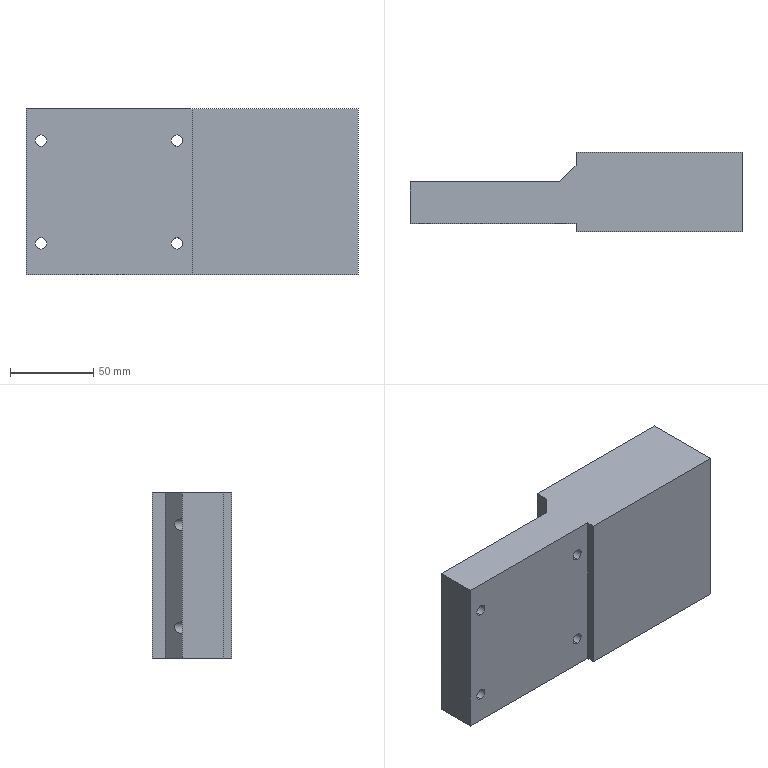Part | STEP file | HXGR200008-05-11 | 1 solid | 35 faces | box 200 x 48 x 100 mm | volume 720235 mm3 | cylinder 16 | plane 11 | cone 8 | commonest cylinder face diameters 6.8 x8 10.2 x8
STEP:
#1=CARTESIAN_POINT('',(115.,15.25,-40.1));
#2=VERTEX_POINT('',#1);
#3=CARTESIAN_POINT('',(115.,15.25,-29.9));
#4=VERTEX_POINT('',#3);
#5=CARTESIAN_POINT('',(115.,15.25,-35.));
#6=DIRECTION('',(0.,1.,0.));
#7=DIRECTION('',(0.,0.,1.));
#8=AXIS2_PLACEMENT_3D('',#5,#6,#7);
#9=CIRCLE('',#8,5.1);
#10=EDGE_CURVE('',#2,#4,#9,.T.);
#11=ORIENTED_EDGE('',*,*,#10,.F.);
#12=CARTESIAN_POINT('',(115.,48.,-40.1));
#13=VERTEX_POINT('',#12);
#14=CARTESIAN_POINT('',(115.,48.,-40.1));
#15=DIRECTION('',(0.,1.,0.));
#16=VECTOR('',#15,1000.);
#17=LINE('',#14,#16);
#18=EDGE_CURVE('',#2,#13,#17,.T.);
#19=ORIENTED_EDGE('',*,*,#18,.T.);
#20=CARTESIAN_POINT('',(115.,48.,-29.9));
#21=VERTEX_POINT('',#20);
#22=CARTESIAN_POINT('',(115.,48.,-35.));
#23=DIRECTION('',(0.,1.,0.));
#24=DIRECTION('',(0.,0.,1.));
#25=AXIS2_PLACEMENT_3D('',#22,#23,#24);
#26=CIRCLE('',#25,5.1);
#27=EDGE_CURVE('',#13,#21,#26,.T.);
#28=ORIENTED_EDGE('',*,*,#27,.T.);
#29=CARTESIAN_POINT('',(115.,48.,-29.9));
#30=DIRECTION('',(0.,1.,0.));
#31=VECTOR('',#30,1000.);
#32=LINE('',#29,#31);
#33=EDGE_CURVE('',#4,#21,#32,.T.);
#34=ORIENTED_EDGE('',*,*,#33,.F.);
#35=EDGE_LOOP('',(#11,#19,#28,#34));
#36=FACE_OUTER_BOUND('',#35,.T.);
#37=CARTESIAN_POINT('',(115.,48.,-35.));
#38=DIRECTION('',(0.,1.,0.));
#39=DIRECTION('',(0.,0.,1.));
#40=AXIS2_PLACEMENT_3D('',#37,#38,#39);
#41=CYLINDRICAL_SURFACE('',#40,5.1);
#42=ADVANCED_FACE('',(#36),#41,.F.);
#43=CARTESIAN_POINT('',(115.,12.186,-35.));
#44=VERTEX_POINT('',#43);
#45=CARTESIAN_POINT('',(115.,15.25,-29.9));
#46=DIRECTION('',(0.,0.515,0.8572));
#47=VECTOR('',#46,1000.);
#48=LINE('',#45,#47);
#49=EDGE_CURVE('',#44,#4,#48,.T.);
#50=ORIENTED_EDGE('',*,*,#49,.F.);
#51=CARTESIAN_POINT('',(115.,15.25,-40.1));
#52=DIRECTION('',(0.,0.515,-0.8572));
#53=VECTOR('',#52,1000.);
#54=LINE('',#51,#53);
#55=EDGE_CURVE('',#44,#2,#54,.T.);
#56=ORIENTED_EDGE('',*,*,#55,.T.);
#57=ORIENTED_EDGE('',*,*,#10,.T.);
#58=EDGE_LOOP('',(#50,#56,#57));
#59=FACE_OUTER_BOUND('',#58,.T.);
#60=CARTESIAN_POINT('',(115.,15.25,-35.));
#61=DIRECTION('',(0.,1.,0.));
#62=DIRECTION('',(0.,0.,1.));
#63=AXIS2_PLACEMENT_3D('',#60,#61,#62);
#64=CONICAL_SURFACE('',#63,5.1,1.03);
#65=ADVANCED_FACE('',(#59),#64,.F.);
#66=CARTESIAN_POINT('',(185.,15.25,-40.1));
#67=VERTEX_POINT('',#66);
#68=CARTESIAN_POINT('',(185.,15.25,-29.9));
#69=VERTEX_POINT('',#68);
#70=CARTESIAN_POINT('',(185.,15.25,-35.));
#71=DIRECTION('',(0.,1.,0.));
#72=DIRECTION('',(0.,0.,1.));
#73=AXIS2_PLACEMENT_3D('',#70,#71,#72);
#74=CIRCLE('',#73,5.1);
#75=EDGE_CURVE('',#67,#69,#74,.T.);
#76=ORIENTED_EDGE('',*,*,#75,.F.);
#77=CARTESIAN_POINT('',(185.,48.,-40.1));
#78=VERTEX_POINT('',#77);
#79=CARTESIAN_POINT('',(185.,48.,-40.1));
#80=DIRECTION('',(0.,1.,0.));
#81=VECTOR('',#80,1000.);
#82=LINE('',#79,#81);
#83=EDGE_CURVE('',#67,#78,#82,.T.);
#84=ORIENTED_EDGE('',*,*,#83,.T.);
#85=CARTESIAN_POINT('',(185.,48.,-29.9));
#86=VERTEX_POINT('',#85);
#87=CARTESIAN_POINT('',(185.,48.,-35.));
#88=DIRECTION('',(0.,1.,0.));
#89=DIRECTION('',(0.,0.,1.));
#90=AXIS2_PLACEMENT_3D('',#87,#88,#89);
#91=CIRCLE('',#90,5.1);
#92=EDGE_CURVE('',#78,#86,#91,.T.);
#93=ORIENTED_EDGE('',*,*,#92,.T.);
#94=CARTESIAN_POINT('',(185.,48.,-29.9));
#95=DIRECTION('',(0.,1.,0.));
#96=VECTOR('',#95,1000.);
#97=LINE('',#94,#96);
#98=EDGE_CURVE('',#69,#86,#97,.T.);
#99=ORIENTED_EDGE('',*,*,#98,.F.);
#100=EDGE_LOOP('',(#76,#84,#93,#99));
#101=FACE_OUTER_BOUND('',#100,.T.);
#102=CARTESIAN_POINT('',(185.,48.,-35.));
#103=DIRECTION('',(0.,1.,0.));
#104=DIRECTION('',(0.,0.,1.));
#105=AXIS2_PLACEMENT_3D('',#102,#103,#104);
#106=CYLINDRICAL_SURFACE('',#105,5.1);
#107=ADVANCED_FACE('',(#101),#106,.F.);
#108=CARTESIAN_POINT('',(185.,12.186,-35.));
#109=VERTEX_POINT('',#108);
#110=CARTESIAN_POINT('',(185.,15.25,-29.9));
#111=DIRECTION('',(0.,0.515,0.8572));
#112=VECTOR('',#111,1000.);
#113=LINE('',#110,#112);
#114=EDGE_CURVE('',#109,#69,#113,.T.);
#115=ORIENTED_EDGE('',*,*,#114,.F.);
#116=CARTESIAN_POINT('',(185.,15.25,-40.1));
#117=DIRECTION('',(0.,0.515,-0.8572));
#118=VECTOR('',#117,1000.);
#119=LINE('',#116,#118);
#120=EDGE_CURVE('',#109,#67,#119,.T.);
#121=ORIENTED_EDGE('',*,*,#120,.T.);
#122=ORIENTED_EDGE('',*,*,#75,.T.);
#123=EDGE_LOOP('',(#115,#121,#122));
#124=FACE_OUTER_BOUND('',#123,.T.);
#125=CARTESIAN_POINT('',(185.,15.25,-35.));
#126=DIRECTION('',(0.,1.,0.));
#127=DIRECTION('',(0.,0.,1.));
#128=AXIS2_PLACEMENT_3D('',#125,#126,#127);
#129=CONICAL_SURFACE('',#128,5.1,1.03);
#130=ADVANCED_FACE('',(#124),#129,.F.);
#131=CARTESIAN_POINT('',(185.,15.25,29.9));
#132=VERTEX_POINT('',#131);
#133=CARTESIAN_POINT('',(185.,15.25,40.1));
#134=VERTEX_POINT('',#133);
#135=CARTESIAN_POINT('',(185.,15.25,35.));
#136=DIRECTION('',(0.,1.,0.));
#137=DIRECTION('',(0.,0.,1.));
#138=AXIS2_PLACEMENT_3D('',#135,#136,#137);
#139=CIRCLE('',#138,5.1);
#140=EDGE_CURVE('',#132,#134,#139,.T.);
#141=ORIENTED_EDGE('',*,*,#140,.F.);
#142=CARTESIAN_POINT('',(185.,48.,29.9));
#143=VERTEX_POINT('',#142);
#144=CARTESIAN_POINT('',(185.,48.,29.9));
#145=DIRECTION('',(0.,1.,0.));
#146=VECTOR('',#145,1000.);
#147=LINE('',#144,#146);
#148=EDGE_CURVE('',#132,#143,#147,.T.);
#149=ORIENTED_EDGE('',*,*,#148,.T.);
#150=CARTESIAN_POINT('',(185.,48.,40.1));
#151=VERTEX_POINT('',#150);
#152=CARTESIAN_POINT('',(185.,48.,35.));
#153=DIRECTION('',(0.,1.,0.));
#154=DIRECTION('',(0.,0.,1.));
#155=AXIS2_PLACEMENT_3D('',#152,#153,#154);
#156=CIRCLE('',#155,5.1);
#157=EDGE_CURVE('',#143,#151,#156,.T.);
#158=ORIENTED_EDGE('',*,*,#157,.T.);
#159=CARTESIAN_POINT('',(185.,48.,40.1));
#160=DIRECTION('',(0.,1.,0.));
#161=VECTOR('',#160,1000.);
#162=LINE('',#159,#161);
#163=EDGE_CURVE('',#134,#151,#162,.T.);
#164=ORIENTED_EDGE('',*,*,#163,.F.);
#165=EDGE_LOOP('',(#141,#149,#158,#164));
#166=FACE_OUTER_BOUND('',#165,.T.);
#167=CARTESIAN_POINT('',(185.,48.,35.));
#168=DIRECTION('',(0.,1.,0.));
#169=DIRECTION('',(0.,0.,1.));
#170=AXIS2_PLACEMENT_3D('',#167,#168,#169);
#171=CYLINDRICAL_SURFACE('',#170,5.1);
#172=ADVANCED_FACE('',(#166),#171,.F.);
#173=CARTESIAN_POINT('',(185.,12.186,35.));
#174=VERTEX_POINT('',#173);
#175=CARTESIAN_POINT('',(185.,15.25,40.1));
#176=DIRECTION('',(0.,0.515,0.8572));
#177=VECTOR('',#176,1000.);
#178=LINE('',#175,#177);
#179=EDGE_CURVE('',#174,#134,#178,.T.);
#180=ORIENTED_EDGE('',*,*,#179,.F.);
#181=CARTESIAN_POINT('',(185.,15.25,29.9));
#182=DIRECTION('',(0.,0.515,-0.8572));
#183=VECTOR('',#182,1000.);
#184=LINE('',#181,#183);
#185=EDGE_CURVE('',#174,#132,#184,.T.);
#186=ORIENTED_EDGE('',*,*,#185,.T.);
#187=ORIENTED_EDGE('',*,*,#140,.T.);
#188=EDGE_LOOP('',(#180,#186,#187));
#189=FACE_OUTER_BOUND('',#188,.T.);
#190=CARTESIAN_POINT('',(185.,15.25,35.));
#191=DIRECTION('',(0.,1.,0.));
#192=DIRECTION('',(0.,0.,1.));
#193=AXIS2_PLACEMENT_3D('',#190,#191,#192);
#194=CONICAL_SURFACE('',#193,5.1,1.03);
#195=ADVANCED_FACE('',(#189),#194,.F.);
#196=CARTESIAN_POINT('',(115.,15.25,29.9));
#197=VERTEX_POINT('',#196);
#198=CARTESIAN_POINT('',(115.,15.25,40.1));
#199=VERTEX_POINT('',#198);
#200=CARTESIAN_POINT('',(115.,15.25,35.));
#201=DIRECTION('',(0.,1.,0.));
#202=DIRECTION('',(0.,0.,1.));
#203=AXIS2_PLACEMENT_3D('',#200,#201,#202);
#204=CIRCLE('',#203,5.1);
#205=EDGE_CURVE('',#197,#199,#204,.T.);
#206=ORIENTED_EDGE('',*,*,#205,.F.);
#207=CARTESIAN_POINT('',(115.,48.,29.9));
#208=VERTEX_POINT('',#207);
#209=CARTESIAN_POINT('',(115.,48.,29.9));
#210=DIRECTION('',(0.,1.,0.));
#211=VECTOR('',#210,1000.);
#212=LINE('',#209,#211);
#213=EDGE_CURVE('',#197,#208,#212,.T.);
#214=ORIENTED_EDGE('',*,*,#213,.T.);
#215=CARTESIAN_POINT('',(115.,48.,40.1));
#216=VERTEX_POINT('',#215);
#217=CARTESIAN_POINT('',(115.,48.,35.));
#218=DIRECTION('',(0.,1.,0.));
#219=DIRECTION('',(0.,0.,1.));
#220=AXIS2_PLACEMENT_3D('',#217,#218,#219);
#221=CIRCLE('',#220,5.1);
#222=EDGE_CURVE('',#208,#216,#221,.T.);
#223=ORIENTED_EDGE('',*,*,#222,.T.);
#224=CARTESIAN_POINT('',(115.,48.,40.1));
#225=DIRECTION('',(0.,1.,0.));
#226=VECTOR('',#225,1000.);
#227=LINE('',#224,#226);
#228=EDGE_CURVE('',#199,#216,#227,.T.);
#229=ORIENTED_EDGE('',*,*,#228,.F.);
#230=EDGE_LOOP('',(#206,#214,#223,#229));
#231=FACE_OUTER_BOUND('',#230,.T.);
#232=CARTESIAN_POINT('',(115.,48.,35.));
#233=DIRECTION('',(0.,1.,0.));
#234=DIRECTION('',(0.,0.,1.));
#235=AXIS2_PLACEMENT_3D('',#232,#233,#234);
#236=CYLINDRICAL_SURFACE('',#235,5.1);
#237=ADVANCED_FACE('',(#231),#236,.F.);
#238=CARTESIAN_POINT('',(115.,12.186,35.));
#239=VERTEX_POINT('',#238);
#240=CARTESIAN_POINT('',(115.,15.25,40.1));
#241=DIRECTION('',(0.,0.515,0.8572));
#242=VECTOR('',#241,1000.);
#243=LINE('',#240,#242);
#244=EDGE_CURVE('',#239,#199,#243,.T.);
#245=ORIENTED_EDGE('',*,*,#244,.F.);
#246=CARTESIAN_POINT('',(115.,15.25,29.9));
#247=DIRECTION('',(0.,0.515,-0.8572));
#248=VECTOR('',#247,1000.);
#249=LINE('',#246,#248);
#250=EDGE_CURVE('',#239,#197,#249,.T.);
#251=ORIENTED_EDGE('',*,*,#250,.T.);
#252=ORIENTED_EDGE('',*,*,#205,.T.);
#253=EDGE_LOOP('',(#245,#251,#252));
#254=FACE_OUTER_BOUND('',#253,.T.);
#255=CARTESIAN_POINT('',(115.,15.25,35.));
#256=DIRECTION('',(0.,1.,0.));
#257=DIRECTION('',(0.,0.,1.));
#258=AXIS2_PLACEMENT_3D('',#255,#256,#257);
#259=CONICAL_SURFACE('',#258,5.1,1.03);
#260=ADVANCED_FACE('',(#254),#259,.F.);
#261=CARTESIAN_POINT('',(90.,30.,-27.75));
#262=VERTEX_POINT('',#261);
#263=CARTESIAN_POINT('',(91.,31.,-27.6));
#264=VERTEX_POINT('',#263);
#265=CARTESIAN_POINT('',(90.,30.,-27.75));
#266=CARTESIAN_POINT('',(90.325,30.325,-27.651));
#267=CARTESIAN_POINT('',(90.66,30.66,-27.6));
#268=CARTESIAN_POINT('',(91.,31.,-27.6));
#269=(BOUNDED_CURVE()B_SPLINE_CURVE(3,(#265,#266,#267,#268),.UNSPECIFIED.,.F.,.F.)B_SPLINE_CURVE_WITH_KNOTS((4,4),(1.272,1.571),.UNSPECIFIED.)CURVE()GEOMETRIC_REPRESENTATION_ITEM()RATIONAL_B_SPLINE_CURVE((1.,0.9926,0.9926,1.))REPRESENTATION_ITEM(''));
#270=EDGE_CURVE('',#262,#264,#269,.T.);
#271=ORIENTED_EDGE('',*,*,#270,.T.);
#272=CARTESIAN_POINT('',(91.,5.,-27.6));
#273=VERTEX_POINT('',#272);
#274=CARTESIAN_POINT('',(91.,5.,-27.6));
#275=DIRECTION('',(0.,-1.,0.));
#276=VECTOR('',#275,1000.);
#277=LINE('',#274,#276);
#278=EDGE_CURVE('',#264,#273,#277,.T.);
#279=ORIENTED_EDGE('',*,*,#278,.T.);
#280=CARTESIAN_POINT('',(91.,5.,-34.4));
#281=VERTEX_POINT('',#280);
#282=CARTESIAN_POINT('',(91.,5.,-31.));
#283=DIRECTION('',(0.,-1.,0.));
#284=DIRECTION('',(0.,0.,-1.));
#285=AXIS2_PLACEMENT_3D('',#282,#283,#284);
#286=CIRCLE('',#285,3.4);
#287=EDGE_CURVE('',#273,#281,#286,.T.);
#288=ORIENTED_EDGE('',*,*,#287,.T.);
#289=CARTESIAN_POINT('',(91.,31.,-34.4));
#290=VERTEX_POINT('',#289);
#291=CARTESIAN_POINT('',(91.,5.,-34.4));
#292=DIRECTION('',(0.,-1.,0.));
#293=VECTOR('',#292,1000.);
#294=LINE('',#291,#293);
#295=EDGE_CURVE('',#290,#281,#294,.T.);
#296=ORIENTED_EDGE('',*,*,#295,.F.);
#297=CARTESIAN_POINT('',(90.,30.,-34.25));
#298=VERTEX_POINT('',#297);
#299=CARTESIAN_POINT('',(91.,31.,-34.4));
#300=CARTESIAN_POINT('',(90.66,30.66,-34.4));
#301=CARTESIAN_POINT('',(90.325,30.325,-34.349));
#302=CARTESIAN_POINT('',(90.,30.,-34.25));
#303=(BOUNDED_CURVE()B_SPLINE_CURVE(3,(#299,#300,#301,#302),.UNSPECIFIED.,.F.,.T.)B_SPLINE_CURVE_WITH_KNOTS((4,4),(4.712,5.011),.UNSPECIFIED.)CURVE()GEOMETRIC_REPRESENTATION_ITEM()RATIONAL_B_SPLINE_CURVE((1.,0.9926,0.9926,1.))REPRESENTATION_ITEM(''));
#304=EDGE_CURVE('',#290,#298,#303,.T.);
#305=ORIENTED_EDGE('',*,*,#304,.T.);
#306=CARTESIAN_POINT('',(91.,30.,-31.));
#307=DIRECTION('',(0.,-1.,0.));
#308=DIRECTION('',(0.,0.,-1.));
#309=AXIS2_PLACEMENT_3D('',#306,#307,#308);
#310=CIRCLE('',#309,3.4);
#311=EDGE_CURVE('',#262,#298,#310,.T.);
#312=ORIENTED_EDGE('',*,*,#311,.F.);
#313=EDGE_LOOP('',(#271,#279,#288,#296,#305,#312));
#314=FACE_OUTER_BOUND('',#313,.T.);
#315=CARTESIAN_POINT('',(91.,5.,-31.));
#316=DIRECTION('',(0.,-1.,0.));
#317=DIRECTION('',(0.,0.,-1.));
#318=AXIS2_PLACEMENT_3D('',#315,#316,#317);
#319=CYLINDRICAL_SURFACE('',#318,3.4);
#320=ADVANCED_FACE('',(#314),#319,.F.);
#321=CARTESIAN_POINT('',(9.,30.,-27.6));
#322=VERTEX_POINT('',#321);
#323=CARTESIAN_POINT('',(9.,30.,-34.4));
#324=VERTEX_POINT('',#323);
#325=CARTESIAN_POINT('',(9.,30.,-31.));
#326=DIRECTION('',(0.,-1.,0.));
#327=DIRECTION('',(0.,0.,-1.));
#328=AXIS2_PLACEMENT_3D('',#325,#326,#327);
#329=CIRCLE('',#328,3.4);
#330=EDGE_CURVE('',#322,#324,#329,.T.);
#331=ORIENTED_EDGE('',*,*,#330,.F.);
#332=CARTESIAN_POINT('',(9.,5.,-27.6));
#333=VERTEX_POINT('',#332);
#334=CARTESIAN_POINT('',(9.,5.,-27.6));
#335=DIRECTION('',(0.,-1.,0.));
#336=VECTOR('',#335,1000.);
#337=LINE('',#334,#336);
#338=EDGE_CURVE('',#322,#333,#337,.T.);
#339=ORIENTED_EDGE('',*,*,#338,.T.);
#340=CARTESIAN_POINT('',(9.,5.,-34.4));
#341=VERTEX_POINT('',#340);
#342=CARTESIAN_POINT('',(9.,5.,-31.));
#343=DIRECTION('',(0.,-1.,0.));
#344=DIRECTION('',(0.,0.,-1.));
#345=AXIS2_PLACEMENT_3D('',#342,#343,#344);
#346=CIRCLE('',#345,3.4);
#347=EDGE_CURVE('',#333,#341,#346,.T.);
#348=ORIENTED_EDGE('',*,*,#347,.T.);
#349=CARTESIAN_POINT('',(9.,5.,-34.4));
#350=DIRECTION('',(0.,-1.,0.));
#351=VECTOR('',#350,1000.);
#352=LINE('',#349,#351);
#353=EDGE_CURVE('',#324,#341,#352,.T.);
#354=ORIENTED_EDGE('',*,*,#353,.F.);
#355=EDGE_LOOP('',(#331,#339,#348,#354));
#356=FACE_OUTER_BOUND('',#355,.T.);
#357=CARTESIAN_POINT('',(9.,5.,-31.));
#358=DIRECTION('',(0.,-1.,0.));
#359=DIRECTION('',(0.,0.,-1.));
#360=AXIS2_PLACEMENT_3D('',#357,#358,#359);
#361=CYLINDRICAL_SURFACE('',#360,3.4);
#362=ADVANCED_FACE('',(#356),#361,.F.);
#363=CARTESIAN_POINT('',(9.,30.,34.4));
#364=VERTEX_POINT('',#363);
#365=CARTESIAN_POINT('',(9.,30.,27.6));
#366=VERTEX_POINT('',#365);
#367=CARTESIAN_POINT('',(9.,30.,31.));
#368=DIRECTION('',(0.,-1.,0.));
#369=DIRECTION('',(0.,0.,-1.));
#370=AXIS2_PLACEMENT_3D('',#367,#368,#369);
#371=CIRCLE('',#370,3.4);
#372=EDGE_CURVE('',#364,#366,#371,.T.);
#373=ORIENTED_EDGE('',*,*,#372,.F.);
#374=CARTESIAN_POINT('',(9.,5.,34.4));
#375=VERTEX_POINT('',#374);
#376=CARTESIAN_POINT('',(9.,5.,34.4));
#377=DIRECTION('',(0.,-1.,0.));
#378=VECTOR('',#377,1000.);
#379=LINE('',#376,#378);
#380=EDGE_CURVE('',#364,#375,#379,.T.);
#381=ORIENTED_EDGE('',*,*,#380,.T.);
#382=CARTESIAN_POINT('',(9.,5.,27.6));
#383=VERTEX_POINT('',#382);
#384=CARTESIAN_POINT('',(9.,5.,31.));
#385=DIRECTION('',(0.,-1.,0.));
#386=DIRECTION('',(0.,0.,-1.));
#387=AXIS2_PLACEMENT_3D('',#384,#385,#386);
#388=CIRCLE('',#387,3.4);
#389=EDGE_CURVE('',#375,#383,#388,.T.);
#390=ORIENTED_EDGE('',*,*,#389,.T.);
#391=CARTESIAN_POINT('',(9.,5.,27.6));
#392=DIRECTION('',(0.,-1.,0.));
#393=VECTOR('',#392,1000.);
#394=LINE('',#391,#393);
#395=EDGE_CURVE('',#366,#383,#394,.T.);
#396=ORIENTED_EDGE('',*,*,#395,.F.);
#397=EDGE_LOOP('',(#373,#381,#390,#396));
#398=FACE_OUTER_BOUND('',#397,.T.);
#399=CARTESIAN_POINT('',(9.,5.,31.));
#400=DIRECTION('',(0.,-1.,0.));
#401=DIRECTION('',(0.,0.,-1.));
#402=AXIS2_PLACEMENT_3D('',#399,#400,#401);
#403=CYLINDRICAL_SURFACE('',#402,3.4);
#404=ADVANCED_FACE('',(#398),#403,.F.);
#405=CARTESIAN_POINT('',(90.,30.,34.25));
#406=VERTEX_POINT('',#405);
#407=CARTESIAN_POINT('',(91.,31.,34.4));
#408=VERTEX_POINT('',#407);
#409=CARTESIAN_POINT('',(90.,30.,34.25));
#410=CARTESIAN_POINT('',(90.325,30.325,34.349));
#411=CARTESIAN_POINT('',(90.66,30.66,34.4));
#412=CARTESIAN_POINT('',(91.,31.,34.4));
#413=(BOUNDED_CURVE()B_SPLINE_CURVE(3,(#409,#410,#411,#412),.UNSPECIFIED.,.F.,.F.)B_SPLINE_CURVE_WITH_KNOTS((4,4),(1.272,1.571),.UNSPECIFIED.)CURVE()GEOMETRIC_REPRESENTATION_ITEM()RATIONAL_B_SPLINE_CURVE((1.,0.9926,0.9926,1.))REPRESENTATION_ITEM(''));
#414=EDGE_CURVE('',#406,#408,#413,.T.);
#415=ORIENTED_EDGE('',*,*,#414,.T.);
#416=CARTESIAN_POINT('',(91.,5.,34.4));
#417=VERTEX_POINT('',#416);
#418=CARTESIAN_POINT('',(91.,5.,34.4));
#419=DIRECTION('',(0.,-1.,0.));
#420=VECTOR('',#419,1000.);
#421=LINE('',#418,#420);
#422=EDGE_CURVE('',#408,#417,#421,.T.);
#423=ORIENTED_EDGE('',*,*,#422,.T.);
#424=CARTESIAN_POINT('',(91.,5.,27.6));
#425=VERTEX_POINT('',#424);
#426=CARTESIAN_POINT('',(91.,5.,31.));
#427=DIRECTION('',(0.,-1.,0.));
#428=DIRECTION('',(0.,0.,-1.));
#429=AXIS2_PLACEMENT_3D('',#426,#427,#428);
#430=CIRCLE('',#429,3.4);
#431=EDGE_CURVE('',#417,#425,#430,.T.);
#432=ORIENTED_EDGE('',*,*,#431,.T.);
#433=CARTESIAN_POINT('',(91.,31.,27.6));
#434=VERTEX_POINT('',#433);
#435=CARTESIAN_POINT('',(91.,5.,27.6));
#436=DIRECTION('',(0.,-1.,0.));
#437=VECTOR('',#436,1000.);
#438=LINE('',#435,#437);
#439=EDGE_CURVE('',#434,#425,#438,.T.);
#440=ORIENTED_EDGE('',*,*,#439,.F.);
#441=CARTESIAN_POINT('',(90.,30.,27.75));
#442=VERTEX_POINT('',#441);
#443=CARTESIAN_POINT('',(91.,31.,27.6));
#444=CARTESIAN_POINT('',(90.66,30.66,27.6));
#445=CARTESIAN_POINT('',(90.325,30.325,27.651));
#446=CARTESIAN_POINT('',(90.,30.,27.75));
#447=(BOUNDED_CURVE()B_SPLINE_CURVE(3,(#443,#444,#445,#446),.UNSPECIFIED.,.F.,.F.)B_SPLINE_CURVE_WITH_KNOTS((4,4),(4.712,5.011),.UNSPECIFIED.)CURVE()GEOMETRIC_REPRESENTATION_ITEM()RATIONAL_B_SPLINE_CURVE((1.,0.9926,0.9926,1.))REPRESENTATION_ITEM(''));
#448=EDGE_CURVE('',#434,#442,#447,.T.);
#449=ORIENTED_EDGE('',*,*,#448,.T.);
#450=CARTESIAN_POINT('',(91.,30.,31.));
#451=DIRECTION('',(0.,-1.,0.));
#452=DIRECTION('',(0.,0.,-1.));
#453=AXIS2_PLACEMENT_3D('',#450,#451,#452);
#454=CIRCLE('',#453,3.4);
#455=EDGE_CURVE('',#406,#442,#454,.T.);
#456=ORIENTED_EDGE('',*,*,#455,.F.);
#457=EDGE_LOOP('',(#415,#423,#432,#440,#449,#456));
#458=FACE_OUTER_BOUND('',#457,.T.);
#459=CARTESIAN_POINT('',(91.,5.,31.));
#460=DIRECTION('',(0.,-1.,0.));
#461=DIRECTION('',(0.,0.,-1.));
#462=AXIS2_PLACEMENT_3D('',#459,#460,#461);
#463=CYLINDRICAL_SURFACE('',#462,3.4);
#464=ADVANCED_FACE('',(#458),#463,.F.);
#465=CARTESIAN_POINT('',(100.,0.,50.));
#466=VERTEX_POINT('',#465);
#467=CARTESIAN_POINT('',(200.,0.,50.));
#468=VERTEX_POINT('',#467);
#469=CARTESIAN_POINT('',(200.,0.,50.));
#470=DIRECTION('',(1.,0.,0.));
#471=VECTOR('',#470,1000.);
#472=LINE('',#469,#471);
#473=EDGE_CURVE('',#466,#468,#472,.T.);
#474=ORIENTED_EDGE('',*,*,#473,.F.);
#475=CARTESIAN_POINT('',(100.,0.,-50.));
#476=VERTEX_POINT('',#475);
#477=CARTESIAN_POINT('',(100.,0.,50.));
#478=DIRECTION('',(0.,0.,-1.));
#479=VECTOR('',#478,1000.);
#480=LINE('',#477,#479);
#481=EDGE_CURVE('',#466,#476,#480,.T.);
#482=ORIENTED_EDGE('',*,*,#481,.T.);
#483=CARTESIAN_POINT('',(200.,0.,-50.));
#484=VERTEX_POINT('',#483);
#485=CARTESIAN_POINT('',(200.,0.,-50.));
#486=DIRECTION('',(1.,0.,0.));
#487=VECTOR('',#486,1000.);
#488=LINE('',#485,#487);
#489=EDGE_CURVE('',#476,#484,#488,.T.);
#490=ORIENTED_EDGE('',*,*,#489,.T.);
#491=CARTESIAN_POINT('',(200.,0.,50.));
#492=DIRECTION('',(0.,0.,-1.));
#493=VECTOR('',#492,1000.);
#494=LINE('',#491,#493);
#495=EDGE_CURVE('',#468,#484,#494,.T.);
#496=ORIENTED_EDGE('',*,*,#495,.F.);
#497=EDGE_LOOP('',(#474,#482,#490,#496));
#498=FACE_OUTER_BOUND('',#497,.T.);
#499=CARTESIAN_POINT('',(200.,0.,50.));
#500=DIRECTION('',(0.,1.,0.));
#501=DIRECTION('',(-1.,0.,0.));
#502=AXIS2_PLACEMENT_3D('',#499,#500,#501);
#503=PLANE('',#502);
#504=ADVANCED_FACE('',(#498),#503,.F.);
#505=CARTESIAN_POINT('',(200.,48.,-50.));
#506=VERTEX_POINT('',#505);
#507=CARTESIAN_POINT('',(200.,48.,-50.));
#508=DIRECTION('',(0.,1.,0.));
#509=VECTOR('',#508,1000.);
#510=LINE('',#507,#509);
#511=EDGE_CURVE('',#484,#506,#510,.T.);
#512=ORIENTED_EDGE('',*,*,#511,.T.);
#513=CARTESIAN_POINT('',(200.,48.,50.));
#514=VERTEX_POINT('',#513);
#515=CARTESIAN_POINT('',(200.,48.,50.));
#516=DIRECTION('',(0.,0.,-1.));
#517=VECTOR('',#516,1000.);
#518=LINE('',#515,#517);
#519=EDGE_CURVE('',#514,#506,#518,.T.);
#520=ORIENTED_EDGE('',*,*,#519,.F.);
#521=CARTESIAN_POINT('',(200.,48.,50.));
#522=DIRECTION('',(0.,1.,0.));
#523=VECTOR('',#522,1000.);
#524=LINE('',#521,#523);
#525=EDGE_CURVE('',#468,#514,#524,.T.);
#526=ORIENTED_EDGE('',*,*,#525,.F.);
#527=ORIENTED_EDGE('',*,*,#495,.T.);
#528=EDGE_LOOP('',(#512,#520,#526,#527));
#529=FACE_OUTER_BOUND('',#528,.T.);
#530=CARTESIAN_POINT('',(200.,48.,50.));
#531=DIRECTION('',(-1.,0.,0.));
#532=DIRECTION('',(0.,0.,1.));
#533=AXIS2_PLACEMENT_3D('',#530,#531,#532);
#534=PLANE('',#533);
#535=ADVANCED_FACE('',(#529),#534,.F.);
#536=CARTESIAN_POINT('',(115.,48.,-35.));
#537=DIRECTION('',(0.,1.,0.));
#538=DIRECTION('',(0.,0.,1.));
#539=AXIS2_PLACEMENT_3D('',#536,#537,#538);
#540=CIRCLE('',#539,5.1);
#541=EDGE_CURVE('',#21,#13,#540,.T.);
#542=ORIENTED_EDGE('',*,*,#541,.F.);
#543=ORIENTED_EDGE('',*,*,#27,.F.);
#544=EDGE_LOOP('',(#542,#543));
#545=FACE_BOUND('',#544,.T.);
#546=CARTESIAN_POINT('',(185.,48.,-35.));
#547=DIRECTION('',(0.,1.,0.));
#548=DIRECTION('',(0.,0.,1.));
#549=AXIS2_PLACEMENT_3D('',#546,#547,#548);
#550=CIRCLE('',#549,5.1);
#551=EDGE_CURVE('',#86,#78,#550,.T.);
#552=ORIENTED_EDGE('',*,*,#551,.F.);
#553=ORIENTED_EDGE('',*,*,#92,.F.);
#554=EDGE_LOOP('',(#552,#553));
#555=FACE_BOUND('',#554,.T.);
#556=CARTESIAN_POINT('',(185.,48.,35.));
#557=DIRECTION('',(0.,1.,0.));
#558=DIRECTION('',(0.,0.,1.));
#559=AXIS2_PLACEMENT_3D('',#556,#557,#558);
#560=CIRCLE('',#559,5.1);
#561=EDGE_CURVE('',#151,#143,#560,.T.);
#562=ORIENTED_EDGE('',*,*,#561,.F.);
#563=ORIENTED_EDGE('',*,*,#157,.F.);
#564=EDGE_LOOP('',(#562,#563));
#565=FACE_BOUND('',#564,.T.);
#566=CARTESIAN_POINT('',(115.,48.,35.));
#567=DIRECTION('',(0.,1.,0.));
#568=DIRECTION('',(0.,0.,1.));
#569=AXIS2_PLACEMENT_3D('',#566,#567,#568);
#570=CIRCLE('',#569,5.1);
#571=EDGE_CURVE('',#216,#208,#570,.T.);
#572=ORIENTED_EDGE('',*,*,#571,.F.);
#573=ORIENTED_EDGE('',*,*,#222,.F.);
#574=EDGE_LOOP('',(#572,#573));
#575=FACE_BOUND('',#574,.T.);
#576=CARTESIAN_POINT('',(100.,48.,-50.));
#577=VERTEX_POINT('',#576);
#578=CARTESIAN_POINT('',(100.,48.,-50.));
#579=DIRECTION('',(-1.,0.,0.));
#580=VECTOR('',#579,1000.);
#581=LINE('',#578,#580);
#582=EDGE_CURVE('',#506,#577,#581,.T.);
#583=ORIENTED_EDGE('',*,*,#582,.T.);
#584=CARTESIAN_POINT('',(100.,48.,50.));
#585=VERTEX_POINT('',#584);
#586=CARTESIAN_POINT('',(100.,48.,50.));
#587=DIRECTION('',(0.,0.,-1.));
#588=VECTOR('',#587,1000.);
#589=LINE('',#586,#588);
#590=EDGE_CURVE('',#585,#577,#589,.T.);
#591=ORIENTED_EDGE('',*,*,#590,.F.);
#592=CARTESIAN_POINT('',(100.,48.,50.));
#593=DIRECTION('',(-1.,0.,0.));
#594=VECTOR('',#593,1000.);
#595=LINE('',#592,#594);
#596=EDGE_CURVE('',#514,#585,#595,.T.);
#597=ORIENTED_EDGE('',*,*,#596,.F.);
#598=ORIENTED_EDGE('',*,*,#519,.T.);
#599=EDGE_LOOP('',(#583,#591,#597,#598));
#600=FACE_OUTER_BOUND('',#599,.T.);
#601=CARTESIAN_POINT('',(100.,48.,50.));
#602=DIRECTION('',(0.,-1.,0.));
#603=DIRECTION('',(1.,0.,0.));
#604=AXIS2_PLACEMENT_3D('',#601,#602,#603);
#605=PLANE('',#604);
#606=ADVANCED_FACE('',(#545,#555,#565,#575,#600),#605,.F.);
#607=CARTESIAN_POINT('',(100.,40.,-50.));
#608=VERTEX_POINT('',#607);
#609=CARTESIAN_POINT('',(100.,30.,-50.));
#610=DIRECTION('',(0.,-1.,0.));
#611=VECTOR('',#610,1000.);
#612=LINE('',#609,#611);
#613=EDGE_CURVE('',#577,#608,#612,.T.);
#614=ORIENTED_EDGE('',*,*,#613,.T.);
#615=CARTESIAN_POINT('',(100.,40.,50.));
#616=VERTEX_POINT('',#615);
#617=CARTESIAN_POINT('',(100.,40.,50.));
#618=DIRECTION('',(0.,0.,1.));
#619=VECTOR('',#618,1000.);
#620=LINE('',#617,#619);
#621=EDGE_CURVE('',#608,#616,#620,.T.);
#622=ORIENTED_EDGE('',*,*,#621,.T.);
#623=CARTESIAN_POINT('',(100.,30.,50.));
#624=DIRECTION('',(0.,-1.,0.));
#625=VECTOR('',#624,1000.);
#626=LINE('',#623,#625);
#627=EDGE_CURVE('',#585,#616,#626,.T.);
#628=ORIENTED_EDGE('',*,*,#627,.F.);
#629=ORIENTED_EDGE('',*,*,#590,.T.);
#630=EDGE_LOOP('',(#614,#622,#628,#629));
#631=FACE_OUTER_BOUND('',#630,.T.);
#632=CARTESIAN_POINT('',(100.,30.,50.));
#633=DIRECTION('',(1.,0.,0.));
#634=DIRECTION('',(0.,0.,-1.));
#635=AXIS2_PLACEMENT_3D('',#632,#633,#634);
#636=PLANE('',#635);
#637=ADVANCED_FACE('',(#631),#636,.F.);
#638=CARTESIAN_POINT('',(9.,30.,-31.));
#639=DIRECTION('',(0.,-1.,0.));
#640=DIRECTION('',(0.,0.,-1.));
#641=AXIS2_PLACEMENT_3D('',#638,#639,#640);
#642=CIRCLE('',#641,3.4);
#643=EDGE_CURVE('',#324,#322,#642,.T.);
#644=ORIENTED_EDGE('',*,*,#643,.T.);
#645=ORIENTED_EDGE('',*,*,#330,.T.);
#646=EDGE_LOOP('',(#644,#645));
#647=FACE_BOUND('',#646,.T.);
#648=CARTESIAN_POINT('',(9.,30.,31.));
#649=DIRECTION('',(0.,-1.,0.));
#650=DIRECTION('',(0.,0.,-1.));
#651=AXIS2_PLACEMENT_3D('',#648,#649,#650);
#652=CIRCLE('',#651,3.4);
#653=EDGE_CURVE('',#366,#364,#652,.T.);
#654=ORIENTED_EDGE('',*,*,#653,.T.);
#655=ORIENTED_EDGE('',*,*,#372,.T.);
#656=EDGE_LOOP('',(#654,#655));
#657=FACE_BOUND('',#656,.T.);
#658=CARTESIAN_POINT('',(90.,30.,50.));
#659=VERTEX_POINT('',#658);
#660=CARTESIAN_POINT('',(0.,30.,50.));
#661=VERTEX_POINT('',#660);
#662=CARTESIAN_POINT('',(0.,30.,50.));
#663=DIRECTION('',(-1.,0.,0.));
#664=VECTOR('',#663,1000.);
#665=LINE('',#662,#664);
#666=EDGE_CURVE('',#659,#661,#665,.T.);
#667=ORIENTED_EDGE('',*,*,#666,.F.);
#668=CARTESIAN_POINT('',(90.,30.,-50.));
#669=DIRECTION('',(0.,0.,-1.));
#670=VECTOR('',#669,1000.);
#671=LINE('',#668,#670);
#672=EDGE_CURVE('',#659,#406,#671,.T.);
#673=ORIENTED_EDGE('',*,*,#672,.T.);
#674=ORIENTED_EDGE('',*,*,#455,.T.);
#675=CARTESIAN_POINT('',(90.,30.,-50.));
#676=DIRECTION('',(0.,0.,-1.));
#677=VECTOR('',#676,1000.);
#678=LINE('',#675,#677);
#679=EDGE_CURVE('',#442,#262,#678,.T.);
#680=ORIENTED_EDGE('',*,*,#679,.T.);
#681=ORIENTED_EDGE('',*,*,#311,.T.);
#682=CARTESIAN_POINT('',(90.,30.,-50.));
#683=VERTEX_POINT('',#682);
#684=CARTESIAN_POINT('',(90.,30.,-50.));
#685=DIRECTION('',(0.,0.,-1.));
#686=VECTOR('',#685,1000.);
#687=LINE('',#684,#686);
#688=EDGE_CURVE('',#298,#683,#687,.T.);
#689=ORIENTED_EDGE('',*,*,#688,.T.);
#690=CARTESIAN_POINT('',(0.,30.,-50.));
#691=VERTEX_POINT('',#690);
#692=CARTESIAN_POINT('',(0.,30.,-50.));
#693=DIRECTION('',(-1.,0.,0.));
#694=VECTOR('',#693,1000.);
#695=LINE('',#692,#694);
#696=EDGE_CURVE('',#683,#691,#695,.T.);
#697=ORIENTED_EDGE('',*,*,#696,.T.);
#698=CARTESIAN_POINT('',(0.,30.,50.));
#699=DIRECTION('',(0.,0.,-1.));
#700=VECTOR('',#699,1000.);
#701=LINE('',#698,#700);
#702=EDGE_CURVE('',#661,#691,#701,.T.);
#703=ORIENTED_EDGE('',*,*,#702,.F.);
#704=EDGE_LOOP('',(#667,#673,#674,#680,#681,#689,#697,#703));
#705=FACE_OUTER_BOUND('',#704,.T.);
#706=CARTESIAN_POINT('',(0.,30.,50.));
#707=DIRECTION('',(0.,-1.,0.));
#708=DIRECTION('',(0.,0.,-1.));
#709=AXIS2_PLACEMENT_3D('',#706,#707,#708);
#710=PLANE('',#709);
#711=ADVANCED_FACE('',(#647,#657,#705),#710,.F.);
#712=CARTESIAN_POINT('',(0.,5.,-50.));
#713=VERTEX_POINT('',#712);
#714=CARTESIAN_POINT('',(0.,0.,-50.));
#715=DIRECTION('',(0.,-1.,0.));
#716=VECTOR('',#715,1000.);
#717=LINE('',#714,#716);
#718=EDGE_CURVE('',#691,#713,#717,.T.);
#719=ORIENTED_EDGE('',*,*,#718,.T.);
#720=CARTESIAN_POINT('',(0.,5.,50.));
#721=VERTEX_POINT('',#720);
#722=CARTESIAN_POINT('',(0.,5.,50.));
#723=DIRECTION('',(0.,0.,-1.));
#724=VECTOR('',#723,1000.);
#725=LINE('',#722,#724);
#726=EDGE_CURVE('',#721,#713,#725,.T.);
#727=ORIENTED_EDGE('',*,*,#726,.F.);
#728=CARTESIAN_POINT('',(0.,0.,50.));
#729=DIRECTION('',(0.,-1.,0.));
#730=VECTOR('',#729,1000.);
#731=LINE('',#728,#730);
#732=EDGE_CURVE('',#661,#721,#731,.T.);
#733=ORIENTED_EDGE('',*,*,#732,.F.);
#734=ORIENTED_EDGE('',*,*,#702,.T.);
#735=EDGE_LOOP('',(#719,#727,#733,#734));
#736=FACE_OUTER_BOUND('',#735,.T.);
#737=CARTESIAN_POINT('',(0.,0.,50.));
#738=DIRECTION('',(1.,0.,0.));
#739=DIRECTION('',(0.,0.,-1.));
#740=AXIS2_PLACEMENT_3D('',#737,#738,#739);
#741=PLANE('',#740);
#742=ADVANCED_FACE('',(#736),#741,.F.);
#743=CARTESIAN_POINT('',(100.,5.,50.));
#744=VERTEX_POINT('',#743);
#745=CARTESIAN_POINT('',(100.,5.,50.));
#746=DIRECTION('',(1.,0.,0.));
#747=VECTOR('',#746,1000.);
#748=LINE('',#745,#747);
#749=EDGE_CURVE('',#721,#744,#748,.T.);
#750=ORIENTED_EDGE('',*,*,#749,.T.);
#751=CARTESIAN_POINT('',(100.,0.,50.));
#752=DIRECTION('',(0.,-1.,0.));
#753=VECTOR('',#752,1000.);
#754=LINE('',#751,#753);
#755=EDGE_CURVE('',#744,#466,#754,.T.);
#756=ORIENTED_EDGE('',*,*,#755,.T.);
#757=ORIENTED_EDGE('',*,*,#473,.T.);
#758=ORIENTED_EDGE('',*,*,#525,.T.);
#759=ORIENTED_EDGE('',*,*,#596,.T.);
#760=ORIENTED_EDGE('',*,*,#627,.T.);
#761=CARTESIAN_POINT('',(30.,-30.,50.));
#762=DIRECTION('',(-0.7071,-0.7071,0.));
#763=VECTOR('',#762,1000.);
#764=LINE('',#761,#763);
#765=EDGE_CURVE('',#616,#659,#764,.T.);
#766=ORIENTED_EDGE('',*,*,#765,.T.);
#767=ORIENTED_EDGE('',*,*,#666,.T.);
#768=ORIENTED_EDGE('',*,*,#732,.T.);
#769=EDGE_LOOP('',(#750,#756,#757,#758,#759,#760,#766,#767,#768));
#770=FACE_OUTER_BOUND('',#769,.T.);
#771=CARTESIAN_POINT('',(0.,0.,50.));
#772=DIRECTION('',(0.,0.,-1.));
#773=DIRECTION('',(-1.,0.,0.));
#774=AXIS2_PLACEMENT_3D('',#771,#772,#773);
#775=PLANE('',#774);
#776=ADVANCED_FACE('',(#770),#775,.F.);
#777=CARTESIAN_POINT('',(100.,5.,-50.));
#778=VERTEX_POINT('',#777);
#779=CARTESIAN_POINT('',(100.,0.,-50.));
#780=DIRECTION('',(0.,-1.,0.));
#781=VECTOR('',#780,1000.);
#782=LINE('',#779,#781);
#783=EDGE_CURVE('',#778,#476,#782,.T.);
#784=ORIENTED_EDGE('',*,*,#783,.F.);
#785=CARTESIAN_POINT('',(100.,5.,-50.));
#786=DIRECTION('',(1.,0.,0.));
#787=VECTOR('',#786,1000.);
#788=LINE('',#785,#787);
#789=EDGE_CURVE('',#713,#778,#788,.T.);
#790=ORIENTED_EDGE('',*,*,#789,.F.);
#791=ORIENTED_EDGE('',*,*,#718,.F.);
#792=ORIENTED_EDGE('',*,*,#696,.F.);
#793=CARTESIAN_POINT('',(90.,30.,-50.));
#794=DIRECTION('',(0.7071,0.7071,0.));
#795=VECTOR('',#794,1000.);
#796=LINE('',#793,#795);
#797=EDGE_CURVE('',#683,#608,#796,.T.);
#798=ORIENTED_EDGE('',*,*,#797,.T.);
#799=ORIENTED_EDGE('',*,*,#613,.F.);
#800=ORIENTED_EDGE('',*,*,#582,.F.);
#801=ORIENTED_EDGE('',*,*,#511,.F.);
#802=ORIENTED_EDGE('',*,*,#489,.F.);
#803=EDGE_LOOP('',(#784,#790,#791,#792,#798,#799,#800,#801,#802));
#804=FACE_OUTER_BOUND('',#803,.T.);
#805=CARTESIAN_POINT('',(0.,0.,-50.));
#806=DIRECTION('',(0.,0.,-1.));
#807=DIRECTION('',(-1.,0.,0.));
#808=AXIS2_PLACEMENT_3D('',#805,#806,#807);
#809=PLANE('',#808);
#810=ADVANCED_FACE('',(#804),#809,.T.);
#811=ORIENTED_EDGE('',*,*,#783,.T.);
#812=ORIENTED_EDGE('',*,*,#481,.F.);
#813=ORIENTED_EDGE('',*,*,#755,.F.);
#814=CARTESIAN_POINT('',(100.,5.,50.));
#815=DIRECTION('',(0.,0.,-1.));
#816=VECTOR('',#815,1000.);
#817=LINE('',#814,#816);
#818=EDGE_CURVE('',#744,#778,#817,.T.);
#819=ORIENTED_EDGE('',*,*,#818,.T.);
#820=EDGE_LOOP('',(#811,#812,#813,#819));
#821=FACE_OUTER_BOUND('',#820,.T.);
#822=CARTESIAN_POINT('',(100.,0.,50.));
#823=DIRECTION('',(1.,0.,0.));
#824=DIRECTION('',(0.,0.,-1.));
#825=AXIS2_PLACEMENT_3D('',#822,#823,#824);
#826=PLANE('',#825);
#827=ADVANCED_FACE('',(#821),#826,.F.);
#828=CARTESIAN_POINT('',(91.,5.,-31.));
#829=DIRECTION('',(0.,-1.,0.));
#830=DIRECTION('',(0.,0.,-1.));
#831=AXIS2_PLACEMENT_3D('',#828,#829,#830);
#832=CIRCLE('',#831,3.4);
#833=EDGE_CURVE('',#281,#273,#832,.T.);
#834=ORIENTED_EDGE('',*,*,#833,.F.);
#835=ORIENTED_EDGE('',*,*,#287,.F.);
#836=EDGE_LOOP('',(#834,#835));
#837=FACE_BOUND('',#836,.T.);
#838=CARTESIAN_POINT('',(9.,5.,-31.));
#839=DIRECTION('',(0.,-1.,0.));
#840=DIRECTION('',(0.,0.,-1.));
#841=AXIS2_PLACEMENT_3D('',#838,#839,#840);
#842=CIRCLE('',#841,3.4);
#843=EDGE_CURVE('',#341,#333,#842,.T.);
#844=ORIENTED_EDGE('',*,*,#843,.F.);
#845=ORIENTED_EDGE('',*,*,#347,.F.);
#846=EDGE_LOOP('',(#844,#845));
#847=FACE_BOUND('',#846,.T.);
#848=CARTESIAN_POINT('',(9.,5.,31.));
#849=DIRECTION('',(0.,-1.,0.));
#850=DIRECTION('',(0.,0.,-1.));
#851=AXIS2_PLACEMENT_3D('',#848,#849,#850);
#852=CIRCLE('',#851,3.4);
#853=EDGE_CURVE('',#383,#375,#852,.T.);
#854=ORIENTED_EDGE('',*,*,#853,.F.);
#855=ORIENTED_EDGE('',*,*,#389,.F.);
#856=EDGE_LOOP('',(#854,#855));
#857=FACE_BOUND('',#856,.T.);
#858=CARTESIAN_POINT('',(91.,5.,31.));
#859=DIRECTION('',(0.,-1.,0.));
#860=DIRECTION('',(0.,0.,-1.));
#861=AXIS2_PLACEMENT_3D('',#858,#859,#860);
#862=CIRCLE('',#861,3.4);
#863=EDGE_CURVE('',#425,#417,#862,.T.);
#864=ORIENTED_EDGE('',*,*,#863,.F.);
#865=ORIENTED_EDGE('',*,*,#431,.F.);
#866=EDGE_LOOP('',(#864,#865));
#867=FACE_BOUND('',#866,.T.);
#868=ORIENTED_EDGE('',*,*,#789,.T.);
#869=ORIENTED_EDGE('',*,*,#818,.F.);
#870=ORIENTED_EDGE('',*,*,#749,.F.);
#871=ORIENTED_EDGE('',*,*,#726,.T.);
#872=EDGE_LOOP('',(#868,#869,#870,#871));
#873=FACE_OUTER_BOUND('',#872,.T.);
#874=CARTESIAN_POINT('',(100.,5.,50.));
#875=DIRECTION('',(0.,1.,0.));
#876=DIRECTION('',(0.,0.,1.));
#877=AXIS2_PLACEMENT_3D('',#874,#875,#876);
#878=PLANE('',#877);
#879=ADVANCED_FACE('',(#837,#847,#857,#867,#873),#878,.F.);
#880=ORIENTED_EDGE('',*,*,#422,.F.);
#881=CARTESIAN_POINT('',(91.,31.,34.4));
#882=CARTESIAN_POINT('',(97.8,37.8,34.4));
#883=CARTESIAN_POINT('',(97.8,37.8,27.6));
#884=CARTESIAN_POINT('',(91.,31.,27.6));
#885=(BOUNDED_CURVE()B_SPLINE_CURVE(3,(#881,#882,#883,#884),.UNSPECIFIED.,.F.,.F.)B_SPLINE_CURVE_WITH_KNOTS((4,4),(1.571,4.712),.UNSPECIFIED.)CURVE()GEOMETRIC_REPRESENTATION_ITEM()RATIONAL_B_SPLINE_CURVE((1.,0.3333,0.3333,1.))REPRESENTATION_ITEM(''));
#886=EDGE_CURVE('',#408,#434,#885,.T.);
#887=ORIENTED_EDGE('',*,*,#886,.T.);
#888=ORIENTED_EDGE('',*,*,#439,.T.);
#889=ORIENTED_EDGE('',*,*,#863,.T.);
#890=EDGE_LOOP('',(#880,#887,#888,#889));
#891=FACE_OUTER_BOUND('',#890,.T.);
#892=CARTESIAN_POINT('',(91.,5.,31.));
#893=DIRECTION('',(0.,-1.,0.));
#894=DIRECTION('',(0.,0.,-1.));
#895=AXIS2_PLACEMENT_3D('',#892,#893,#894);
#896=CYLINDRICAL_SURFACE('',#895,3.4);
#897=ADVANCED_FACE('',(#891),#896,.F.);
#898=ORIENTED_EDGE('',*,*,#380,.F.);
#899=ORIENTED_EDGE('',*,*,#653,.F.);
#900=ORIENTED_EDGE('',*,*,#395,.T.);
#901=ORIENTED_EDGE('',*,*,#853,.T.);
#902=EDGE_LOOP('',(#898,#899,#900,#901));
#903=FACE_OUTER_BOUND('',#902,.T.);
#904=CARTESIAN_POINT('',(9.,5.,31.));
#905=DIRECTION('',(0.,-1.,0.));
#906=DIRECTION('',(0.,0.,-1.));
#907=AXIS2_PLACEMENT_3D('',#904,#905,#906);
#908=CYLINDRICAL_SURFACE('',#907,3.4);
#909=ADVANCED_FACE('',(#903),#908,.F.);
#910=ORIENTED_EDGE('',*,*,#338,.F.);
#911=ORIENTED_EDGE('',*,*,#643,.F.);
#912=ORIENTED_EDGE('',*,*,#353,.T.);
#913=ORIENTED_EDGE('',*,*,#843,.T.);
#914=EDGE_LOOP('',(#910,#911,#912,#913));
#915=FACE_OUTER_BOUND('',#914,.T.);
#916=CARTESIAN_POINT('',(9.,5.,-31.));
#917=DIRECTION('',(0.,-1.,0.));
#918=DIRECTION('',(0.,0.,-1.));
#919=AXIS2_PLACEMENT_3D('',#916,#917,#918);
#920=CYLINDRICAL_SURFACE('',#919,3.4);
#921=ADVANCED_FACE('',(#915),#920,.F.);
#922=ORIENTED_EDGE('',*,*,#278,.F.);
#923=CARTESIAN_POINT('',(91.,31.,-27.6));
#924=CARTESIAN_POINT('',(97.8,37.8,-27.6));
#925=CARTESIAN_POINT('',(97.8,37.8,-34.4));
#926=CARTESIAN_POINT('',(91.,31.,-34.4));
#927=(BOUNDED_CURVE()B_SPLINE_CURVE(3,(#923,#924,#925,#926),.UNSPECIFIED.,.F.,.F.)B_SPLINE_CURVE_WITH_KNOTS((4,4),(1.571,4.712),.UNSPECIFIED.)CURVE()GEOMETRIC_REPRESENTATION_ITEM()RATIONAL_B_SPLINE_CURVE((1.,0.3333,0.3333,1.))REPRESENTATION_ITEM(''));
#928=EDGE_CURVE('',#264,#290,#927,.T.);
#929=ORIENTED_EDGE('',*,*,#928,.T.);
#930=ORIENTED_EDGE('',*,*,#295,.T.);
#931=ORIENTED_EDGE('',*,*,#833,.T.);
#932=EDGE_LOOP('',(#922,#929,#930,#931));
#933=FACE_OUTER_BOUND('',#932,.T.);
#934=CARTESIAN_POINT('',(91.,5.,-31.));
#935=DIRECTION('',(0.,-1.,0.));
#936=DIRECTION('',(0.,0.,-1.));
#937=AXIS2_PLACEMENT_3D('',#934,#935,#936);
#938=CYLINDRICAL_SURFACE('',#937,3.4);
#939=ADVANCED_FACE('',(#933),#938,.F.);
#940=ORIENTED_EDGE('',*,*,#250,.F.);
#941=ORIENTED_EDGE('',*,*,#244,.T.);
#942=CARTESIAN_POINT('',(115.,15.25,35.));
#943=DIRECTION('',(0.,1.,0.));
#944=DIRECTION('',(0.,0.,1.));
#945=AXIS2_PLACEMENT_3D('',#942,#943,#944);
#946=CIRCLE('',#945,5.1);
#947=EDGE_CURVE('',#199,#197,#946,.T.);
#948=ORIENTED_EDGE('',*,*,#947,.T.);
#949=EDGE_LOOP('',(#940,#941,#948));
#950=FACE_OUTER_BOUND('',#949,.T.);
#951=CARTESIAN_POINT('',(115.,15.25,35.));
#952=DIRECTION('',(0.,1.,0.));
#953=DIRECTION('',(0.,0.,1.));
#954=AXIS2_PLACEMENT_3D('',#951,#952,#953);
#955=CONICAL_SURFACE('',#954,5.1,1.03);
#956=ADVANCED_FACE('',(#950),#955,.F.);
#957=ORIENTED_EDGE('',*,*,#213,.F.);
#958=ORIENTED_EDGE('',*,*,#947,.F.);
#959=ORIENTED_EDGE('',*,*,#228,.T.);
#960=ORIENTED_EDGE('',*,*,#571,.T.);
#961=EDGE_LOOP('',(#957,#958,#959,#960));
#962=FACE_OUTER_BOUND('',#961,.T.);
#963=CARTESIAN_POINT('',(115.,48.,35.));
#964=DIRECTION('',(0.,1.,0.));
#965=DIRECTION('',(0.,0.,1.));
#966=AXIS2_PLACEMENT_3D('',#963,#964,#965);
#967=CYLINDRICAL_SURFACE('',#966,5.1);
#968=ADVANCED_FACE('',(#962),#967,.F.);
#969=ORIENTED_EDGE('',*,*,#185,.F.);
#970=ORIENTED_EDGE('',*,*,#179,.T.);
#971=CARTESIAN_POINT('',(185.,15.25,35.));
#972=DIRECTION('',(0.,1.,0.));
#973=DIRECTION('',(0.,0.,1.));
#974=AXIS2_PLACEMENT_3D('',#971,#972,#973);
#975=CIRCLE('',#974,5.1);
#976=EDGE_CURVE('',#134,#132,#975,.T.);
#977=ORIENTED_EDGE('',*,*,#976,.T.);
#978=EDGE_LOOP('',(#969,#970,#977));
#979=FACE_OUTER_BOUND('',#978,.T.);
#980=CARTESIAN_POINT('',(185.,15.25,35.));
#981=DIRECTION('',(0.,1.,0.));
#982=DIRECTION('',(0.,0.,1.));
#983=AXIS2_PLACEMENT_3D('',#980,#981,#982);
#984=CONICAL_SURFACE('',#983,5.1,1.03);
#985=ADVANCED_FACE('',(#979),#984,.F.);
#986=ORIENTED_EDGE('',*,*,#148,.F.);
#987=ORIENTED_EDGE('',*,*,#976,.F.);
#988=ORIENTED_EDGE('',*,*,#163,.T.);
#989=ORIENTED_EDGE('',*,*,#561,.T.);
#990=EDGE_LOOP('',(#986,#987,#988,#989));
#991=FACE_OUTER_BOUND('',#990,.T.);
#992=CARTESIAN_POINT('',(185.,48.,35.));
#993=DIRECTION('',(0.,1.,0.));
#994=DIRECTION('',(0.,0.,1.));
#995=AXIS2_PLACEMENT_3D('',#992,#993,#994);
#996=CYLINDRICAL_SURFACE('',#995,5.1);
#997=ADVANCED_FACE('',(#991),#996,.F.);
#998=ORIENTED_EDGE('',*,*,#120,.F.);
#999=ORIENTED_EDGE('',*,*,#114,.T.);
#1000=CARTESIAN_POINT('',(185.,15.25,-35.));
#1001=DIRECTION('',(0.,1.,0.));
#1002=DIRECTION('',(0.,0.,1.));
#1003=AXIS2_PLACEMENT_3D('',#1000,#1001,#1002);
#1004=CIRCLE('',#1003,5.1);
#1005=EDGE_CURVE('',#69,#67,#1004,.T.);
#1006=ORIENTED_EDGE('',*,*,#1005,.T.);
#1007=EDGE_LOOP('',(#998,#999,#1006));
#1008=FACE_OUTER_BOUND('',#1007,.T.);
#1009=CARTESIAN_POINT('',(185.,15.25,-35.));
#1010=DIRECTION('',(0.,1.,0.));
#1011=DIRECTION('',(0.,0.,1.));
#1012=AXIS2_PLACEMENT_3D('',#1009,#1010,#1011);
#1013=CONICAL_SURFACE('',#1012,5.1,1.03);
#1014=ADVANCED_FACE('',(#1008),#1013,.F.);
#1015=ORIENTED_EDGE('',*,*,#83,.F.);
#1016=ORIENTED_EDGE('',*,*,#1005,.F.);
#1017=ORIENTED_EDGE('',*,*,#98,.T.);
#1018=ORIENTED_EDGE('',*,*,#551,.T.);
#1019=EDGE_LOOP('',(#1015,#1016,#1017,#1018));
#1020=FACE_OUTER_BOUND('',#1019,.T.);
#1021=CARTESIAN_POINT('',(185.,48.,-35.));
#1022=DIRECTION('',(0.,1.,0.));
#1023=DIRECTION('',(0.,0.,1.));
#1024=AXIS2_PLACEMENT_3D('',#1021,#1022,#1023);
#1025=CYLINDRICAL_SURFACE('',#1024,5.1);
#1026=ADVANCED_FACE('',(#1020),#1025,.F.);
#1027=ORIENTED_EDGE('',*,*,#55,.F.);
#1028=ORIENTED_EDGE('',*,*,#49,.T.);
#1029=CARTESIAN_POINT('',(115.,15.25,-35.));
#1030=DIRECTION('',(0.,1.,0.));
#1031=DIRECTION('',(0.,0.,1.));
#1032=AXIS2_PLACEMENT_3D('',#1029,#1030,#1031);
#1033=CIRCLE('',#1032,5.1);
#1034=EDGE_CURVE('',#4,#2,#1033,.T.);
#1035=ORIENTED_EDGE('',*,*,#1034,.T.);
#1036=EDGE_LOOP('',(#1027,#1028,#1035));
#1037=FACE_OUTER_BOUND('',#1036,.T.);
#1038=CARTESIAN_POINT('',(115.,15.25,-35.));
#1039=DIRECTION('',(0.,1.,0.));
#1040=DIRECTION('',(0.,0.,1.));
#1041=AXIS2_PLACEMENT_3D('',#1038,#1039,#1040);
#1042=CONICAL_SURFACE('',#1041,5.1,1.03);
#1043=ADVANCED_FACE('',(#1037),#1042,.F.);
#1044=ORIENTED_EDGE('',*,*,#18,.F.);
#1045=ORIENTED_EDGE('',*,*,#1034,.F.);
#1046=ORIENTED_EDGE('',*,*,#33,.T.);
#1047=ORIENTED_EDGE('',*,*,#541,.T.);
#1048=EDGE_LOOP('',(#1044,#1045,#1046,#1047));
#1049=FACE_OUTER_BOUND('',#1048,.T.);
#1050=CARTESIAN_POINT('',(115.,48.,-35.));
#1051=DIRECTION('',(0.,1.,0.));
#1052=DIRECTION('',(0.,0.,1.));
#1053=AXIS2_PLACEMENT_3D('',#1050,#1051,#1052);
#1054=CYLINDRICAL_SURFACE('',#1053,5.1);
#1055=ADVANCED_FACE('',(#1049),#1054,.F.);
#1056=ORIENTED_EDGE('',*,*,#765,.F.);
#1057=ORIENTED_EDGE('',*,*,#621,.F.);
#1058=ORIENTED_EDGE('',*,*,#797,.F.);
#1059=ORIENTED_EDGE('',*,*,#688,.F.);
#1060=ORIENTED_EDGE('',*,*,#304,.F.);
#1061=ORIENTED_EDGE('',*,*,#928,.F.);
#1062=ORIENTED_EDGE('',*,*,#270,.F.);
#1063=ORIENTED_EDGE('',*,*,#679,.F.);
#1064=ORIENTED_EDGE('',*,*,#448,.F.);
#1065=ORIENTED_EDGE('',*,*,#886,.F.);
#1066=ORIENTED_EDGE('',*,*,#414,.F.);
#1067=ORIENTED_EDGE('',*,*,#672,.F.);
#1068=EDGE_LOOP('',(#1056,#1057,#1058,#1059,#1060,#1061,#1062,#1063,#1064,#1065,#1066,#1067));
#1069=FACE_OUTER_BOUND('',#1068,.T.);
#1070=CARTESIAN_POINT('',(90.,30.,50.));
#1071=DIRECTION('',(-0.7071,0.7071,0.));
#1072=DIRECTION('',(0.,0.,1.));
#1073=AXIS2_PLACEMENT_3D('',#1070,#1071,#1072);
#1074=PLANE('',#1073);
#1075=ADVANCED_FACE('',(#1069),#1074,.T.);
#1076=CLOSED_SHELL('',(#42,#65,#107,#130,#172,#195,#237,#260,#320,#362,#404,#464,#504,#535,#606,#637,#711,#742,#776,#810,#827,#879,#897,#909,#921,#939,#956,#968,#985,#997,#1014,#1026,#1043,#1055,#1075));
#1077=MANIFOLD_SOLID_BREP('',#1076);
#1078=CARTESIAN_POINT('',(0.,0.,0.));
#1079=DIRECTION('',(0.,0.,1.));
#1080=DIRECTION('',(1.,0.,0.));
#1081=AXIS2_PLACEMENT_3D('',#1078,#1079,#1080);
#1082=(LENGTH_UNIT()NAMED_UNIT(*)SI_UNIT(.MILLI.,.METRE.));
#1083=UNCERTAINTY_MEASURE_WITH_UNIT(LENGTH_MEASURE(0.00001),#1082,'','');
#1084=(NAMED_UNIT(*)PLANE_ANGLE_UNIT()SI_UNIT($,.RADIAN.));
#1085=(NAMED_UNIT(*)SI_UNIT($,.STERADIAN.)SOLID_ANGLE_UNIT());
#1086=(GEOMETRIC_REPRESENTATION_CONTEXT(3)GLOBAL_UNCERTAINTY_ASSIGNED_CONTEXT((#1083))GLOBAL_UNIT_ASSIGNED_CONTEXT((#1082,#1084,#1085))REPRESENTATION_CONTEXT('',''));
#1087=ADVANCED_BREP_SHAPE_REPRESENTATION('',(#1077,#1081),#1086);